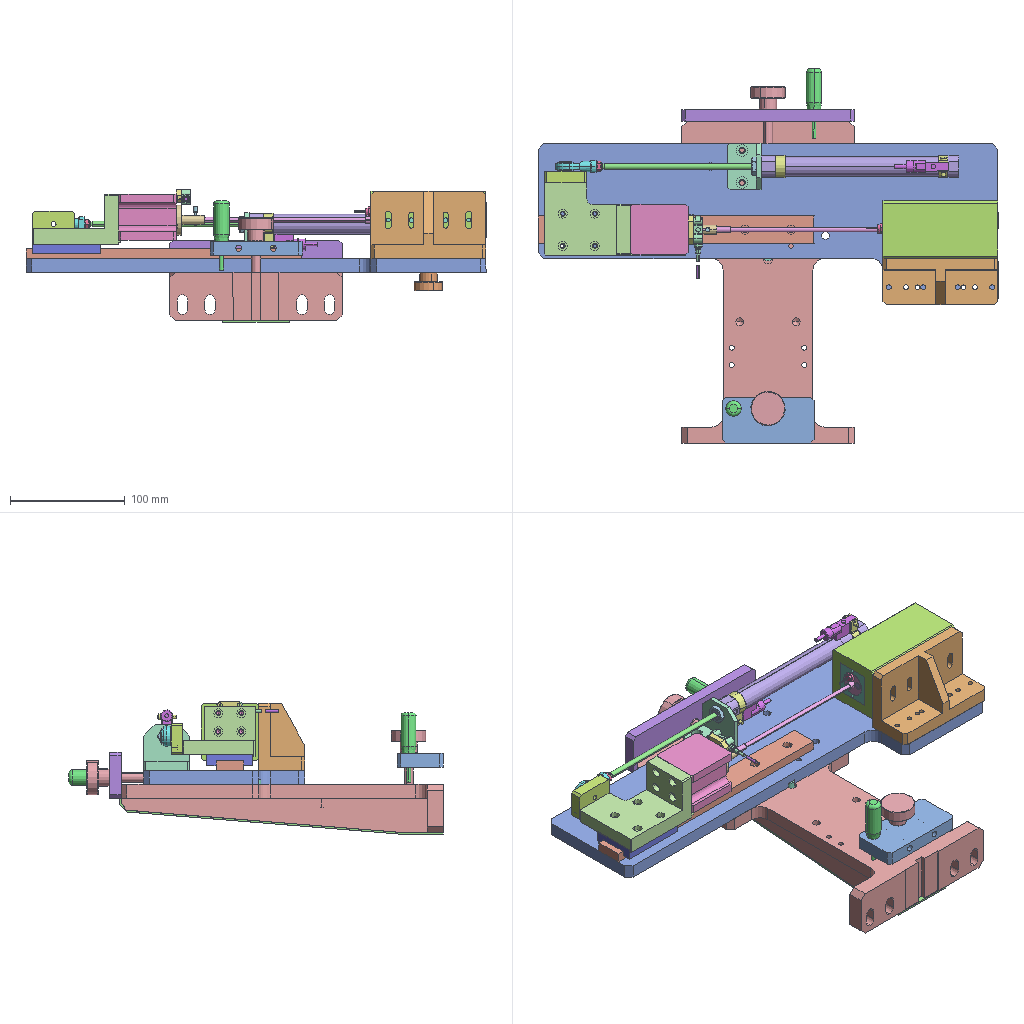Assembly | SolidWorks | 34 different items | 39 placed | box 400 x 326 x 116 mm
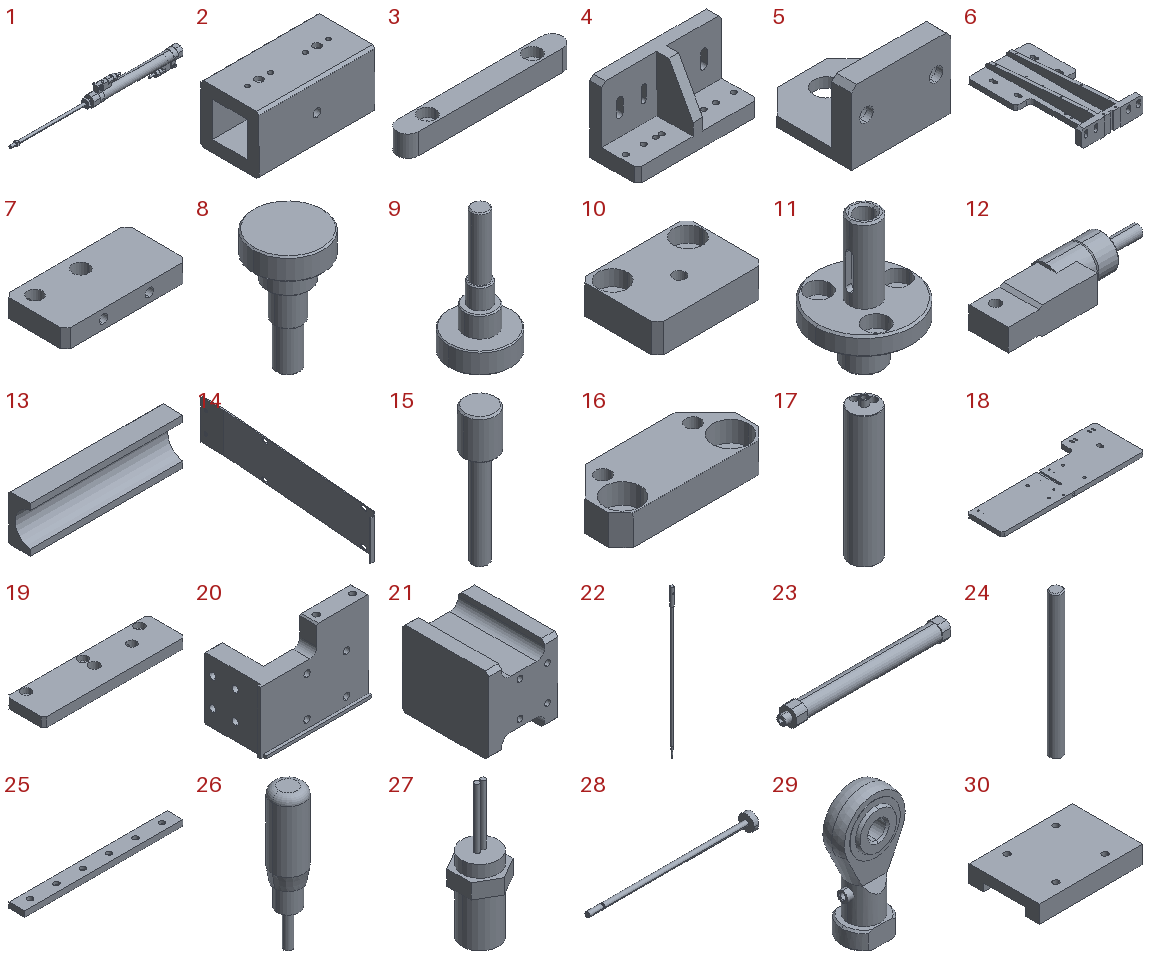Parts list (item | name | quantity | parent item | size | volume | features):
1 | (subassembly) | x1 | - | 325 x 19.2 x 45.4 mm | 28867 mm3 | -
2 | - | x1 | - | 100 x 50 x 50 mm | 157737 mm3 | features HoleWzd 7, Chamfer 1, Extrusion 1, ICE 1
3 | - | x1 | - | 63 x 8 x 8 mm | 3613 mm3 | features Extrusion 1, HoleWzd 1
4 | - | x1 | - | 100 x 40 x 58.5 mm | 98616 mm3 | features ICE 3, Chamfer 1, Extrusion 1, HoleWzd 1, Rib 1
5 | - | x1 | - | 40 x 40 x 29 mm | 12650 mm3 | features Chamfer 2, ICE 2, Extrusion 1, HoleWzd 1
6 | - | x1 | - | 150 x 280 x 42 mm | 505968 mm3 | features HoleWzd 8, ICE 7, Chamfer 3, MirrorPattern 3, Extrusion 1, Fillet 1, Rib 1
7 | - | x1 | - | 80 x 40 x 12 mm | 30513 mm3 | features HoleWzd 2, Chamfer 1, Extrusion 1, ICE 1
8 | - | x1 | - | 25 x 25 x 43 mm | 7005 mm3 | features ICE 3, Chamfer 1, Extrusion 1
9 | - | x2 | - | 30 x 30 x 60 mm | 11093 mm3 | features ICE 3, Chamfer 1, Extrusion 1
10 | - | x1 | - | 37 x 27 x 10 mm | 8705 mm3 | features HoleWzd 2, Chamfer 1, Extrusion 1
11 | - | x1 | - | 26 x 26 x 35 mm | 3387 mm3 | features ICE 4, Chamfer 1, CirPattern 1, Extrusion 1, HoleWzd 1
12 | - | x2 | in 1 | 46.7 x 14 x 10 mm | 3223 mm3 | features ICE 5, RefAxis 3, Revolution 2, 3DProfileFeature 1, Extrusion 1, RevCut 1
13 | - | x2 | - | 100 x 14 x 30 mm | 25090 mm3 | features Chamfer 1, Extrusion 1, ICE 1
14 | - | x1 | - | 31.5 x 281.5 x 58 mm | 24856 mm3 | features ICE 2, ExtruThin 1, MirrorPattern 1
15 | - | x1 | - | 4 x 4 x 17 mm | 99.928 mm3 | features Chamfer 1, Extrusion 1, ICE 1
16 | - | x1 | - | 25 x 11 x 5 mm | 959.594 mm3 | features Chamfer 2, HoleWzd 2, Extrusion 1
17 | - | x1 | - | 22 x 22 x 105 mm | 33982 mm3 | features ICE 3, Chamfer 1, Extrusion 1, HoleWzd 1
18 | - | x1 | - | 400 x 140 x 12 mm | 518070 mm3 | features HoleWzd 5, ICE 5, Chamfer 1, Extrusion 1, Fillet 1
19 | - | x1 | - | 150 x 40 x 10 mm | 56531 mm3 | features HoleWzd 3, Chamfer 1, Extrusion 1, ICE 1
20 | - | x1 | - | 77 x 44 x 63 mm | 61294 mm3 | features ICE 6, HoleWzd 4, Chamfer 1, Extrusion 1, Fillet 1
21 | - | x1 | - | 40 x 50 x 44 mm | 66825 mm3 | features HoleWzd 3, ICE 2, Chamfer 1, CirPattern 1, Extrusion 1, Fillet 1
22 | - | x1 | - | 5 x 5 x 260 mm | 2905 mm3 | features ICE 3, Chamfer 1, Extrusion 1
23 | - | x1 | in 1 | 180 x 18.3 x 18.3 mm | 16108 mm3 | features RefAxis 21, 3DProfileFeature 7, ICE 3, HoleWzd 2, RevCut 1, Revolution 1
24 | - | x1 | - | 6 x 6 x 70 mm | 1975 mm3 | features Chamfer 1, Extrusion 1
25 | - | x1 | - | 240 x 24 x 8.5 mm | 47242 mm3 | features Extrusion 1, HoleWzd 1, LPattern 1
26 | - | x2 | - | 13.5 x 13.5 x 60.5 mm | 5709 mm3 | features ICE 2, Chamfer 1, Extrusion 1, Fillet 1
27 | - | x1 | - | 7 x 8.083 x 22.5 mm | 398.885 mm3 | features ICE 3, Extrusion 1
28 | - | x1 | in 1 | 170.5 x 16 x 16 mm | 4244 mm3 | features RefAxis 9, 3DProfileFeature 3, Revolution 1
29 | - | x1 | - | 18 x 10 x 36 mm | 2766 mm3 | features Revolution 4, ICE 2, RevCut 2
30 | - | x1 | - | 59.4 x 40 x 10 mm | 17003 mm3 | features Extrusion 1, HoleWzd 1, ICE 1
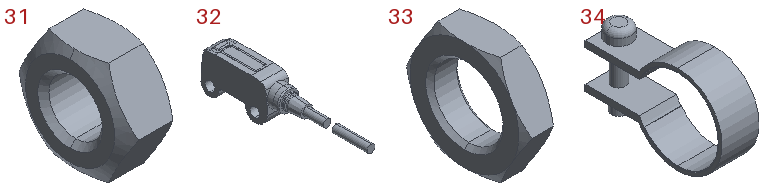31 | - | x1 | in 1 | 4 x 9.238 x 8 mm | 156.615 mm3 | features RefAxis 6, 3DProfileFeature 2, RevCut 2, Extrusion 1
32 | - | x1 | - | 7.5 x 54.319 x 13.3 mm | 2039 mm3 | features BaseBody 2
33 | - | x1 | in 1 | 4 x 16.166 x 14 mm | 414.657 mm3 | features RefAxis 6, 3DProfileFeature 2, RevCut 2, Extrusion 1
34 | - | x2 | in 1 | 8 x 29.6 x 19.2 mm | 748.959 mm3 | features RefAxis 6, 3DProfileFeature 2, Extrusion 1, ICE 1, Revolution 1
Mates (type | each side: item.copy, entity, surface, feature):
In the top assembly
Coincident | 6.1 face plane Boss-Extrude1 | 18.1 face plane Boss-Extrude1
Parallel | 6.1 face plane Boss-Extrude1 | 18.1 face plane Boss-Extrude1
Coincident | 2.1 face plane Boss-Extrude1 | 13.1 face plane Boss-Extrude1
Coincident | 2.1 face plane Cut-Extrude1 | 13.1 face plane Boss-Extrude1
Concentric | 17.1 face cylinder Boss-Extrude1 | 13.2 face cylinder Cut-Extrude1
Coincident | 17.1 face plane Boss-Extrude1 | 13.2 face plane Boss-Extrude1
Coincident | 2.1 face plane Cut-Extrude1 | 13.2 face plane Boss-Extrude1
Coincident | 18.1 face plane Boss-Extrude1 | 4.1 face plane Boss-Extrude1
Coincident | 2.1 face plane Boss-Extrude1 | 4.1 face plane Boss-Extrude1 | 3 times
Coincident | 18.1 face plane Boss-Extrude2 | 4.1 face plane Boss-Extrude1 | 2 times
Parallel | 18.1 face plane Boss-Extrude1 | 23.1 face plane Boss-Extrude1 | 3 times
Concentric | 23.1 face cylinder Revolve1 | 5.1 face cylinder Cut-Extrude1
Coincident | 18.1 face plane Boss-Extrude1 | 5.1 face plane Boss-Extrude1 | 2 times
Coincident | 23.1 face plane Boss-Extrude1 | 5.1 face plane Boss-Extrude1
Parallel | 18.1 face plane Boss-Extrude1 | 5.1 face plane Boss-Extrude1
Coincident | 18.1 face plane Boss-Extrude1 | 25.1 face plane Boss-Extrude1 | 2 times
Parallel | 18.1 face plane Boss-Extrude1 | 25.1 face plane Boss-Extrude1
Coincident | 25.1 face plane Boss-Extrude1 | 30.1 face plane Cut-Extrude1 | 3 times
Coincident | 30.1 face plane Boss-Extrude1 | 20.1 face plane Boss-Extrude1
Width | 25.1 face plane Boss-Extrude1 | 25.1 face plane Boss-Extrude1 | 30.1 face plane Boss-Extrude1 | 30.1 face plane Boss-Extrude1
Coincident | 30.1 face plane Boss-Extrude1 | 20.1 face plane Boss-Extrude2
Coincident | 20.1 face plane Boss-Extrude1 | 21.1 face plane Boss-Extrude1
Coincident | 20.1 face plane Boss-Extrude5 | 21.1 face plane Boss-Extrude1
Coincident | 20.1 face plane Cut-Extrude2 | 21.1 face plane Boss-Extrude1
Concentric | 28.1 face cylinder Revolve1 | 29.1 face cylinder Revolve1
Coincident | 31.1 face plane Boss-Extrude1 | 29.1 face plane Revolve1
DistanceDim | 5.1 face plane Boss-Extrude2 | 18.1 face plane Boss-Extrude1
Concentric | 21.1 face cylinder Cut-Extrude1 | 11.1 face cylinder Boss-Extrude1
Coincident | 21.1 face plane Boss-Extrude1 | 11.1 face plane Boss-Extrude2
Width | 6.1 face plane Boss-Extrude1 | 6.1 face plane Boss-Extrude1 | 18.1 face plane Boss-Extrude1 | 18.1 face plane Boss-Extrude1
Concentric | 21.1 face cylinder CirPattern1 | 11.1 face cylinder CirPattern1
Coincident | 6.1 face plane Boss-Extrude1 | 19.1 face plane Boss-Extrude1 | 3 times
Concentric | 19.1 face cylinder Cut-Extrude1 | 26.1 face cylinder Boss-Extrude2
Coincident | 19.1 face plane Boss-Extrude1 | 26.1 face plane Boss-Extrude3
Concentric | 19.1 face cylinder Ø10.5 (10.5) Diameter Hole1 | 9.1 face cylinder Boss-Extrude2
Coincident | 19.1 face plane Boss-Extrude1 | 9.1 face plane Boss-Extrude2
Width | 6.1 face plane Boss-Extrude1 | 6.1 face plane Boss-Extrude1 | 7.1 face plane Boss-Extrude1 | 7.1 face plane Boss-Extrude1
DistanceDim | 7.1 face plane Boss-Extrude1 | 6.1 face plane Boss-Extrude1
Concentric | 7.1 face cylinder Cut-Extrude1 | 9.2 face cylinder Boss-Extrude4
Coincident | 7.1 face plane Boss-Extrude1 | 9.2 face plane Boss-Extrude2
Concentric | 7.1 face cylinder Cut-Extrude1 | 26.2 face cylinder Boss-Extrude3
Coincident | 7.1 face plane Boss-Extrude1 | 26.2 face plane Boss-Extrude3
Coincident | 6.1 face plane Boss-Extrude1 | 7.1 face plane Boss-Extrude1
DistanceDim | 18.1 face plane Boss-Extrude1 | 6.1 face plane Boss-Extrude1
Width | 25.1 face plane Boss-Extrude1 | 25.1 face plane Boss-Extrude1 | 17.1 face cylinder Boss-Extrude2
Concentric | 20.1 face cylinder M5 Tapped Hole2 | 10.1 face cylinder CBORE for M5 Hex Socket Head Cap Screw1 | 2 times
Coincident | 20.1 face plane Cut-Extrude3 | 10.1 face plane Boss-Extrude1
Coincident | 29.1 face plane Revolve3 | 10.1 face plane Boss-Extrude1
Concentric | 29.1 face cylinder Cut-Revolve1 | 10.1 face cylinder M5 Tapped Hole1
Concentric | 11.1 face cylinder Boss-Extrude3 | 22.1 face cylinder Boss-Extrude2
Concentric | 11.1 face cylinder Cut-Extrude2 | 22.1 face cylinder Cut-Extrude1
Concentric | 30.1 face cylinder M4 Tapped Hole1 | 20.1 face cylinder CBORE for M4 Hex Socket Head Cap Screw2
Coincident | 6.1 face plane Cut-Extrude3 | 3.1 face plane Boss-Extrude1 | 2 times
Concentric | 6.1 face cylinder M3 Tapped Hole1 | 3.1 face cylinder CBORE for M3 Hex Socket Head Cap Screw1
Coincident | 2.1 face plane Boss-Extrude1 | 4.1 face plane Boss-Extrude2
Concentric | 17.1 face cylinder Boss-Extrude1 | 13.1 face cylinder Cut-Extrude1
Coincident | 2.1 face plane Boss-Extrude1 | 13.2 face plane Boss-Extrude1
Concentric | 2.1 face cylinder M8 Tapped Hole1 | 8.1 face cylinder Boss-Extrude2
Coincident | 18.1 face plane Boss-Extrude1 | 8.1 face plane Boss-Extrude3
Coincident | 6.1 face plane Boss-Extrude2 | assembly plane
Coincident | 6.1 face plane Boss-Extrude1 | assembly plane
Coincident | 6.1 face plane Mirror1 | assembly plane
Concentric | 17.1 face cylinder Cut-Extrude2 | 24.1 face cylinder Boss-Extrude1
Coincident | 17.1 face plane Boss-Extrude1 | 24.1 face plane Boss-Extrude1
Coincident | 6.1 face plane Boss-Extrude1 | 14.1 face plane Extrude-Thin2
Coincident | 6.1 face plane Boss-Extrude2 | 14.1 face plane Extrude-Thin2
Coincident | 6.1 face plane Rib1 | 14.1 face plane Extrude-Thin2
Coincident | 17.1 face plane Boss-Extrude1 | 27.1 face plane Boss-Extrude2
Concentric | 17.1 face cylinder M6 Tapped Hole1 | 27.1 face cylinder Boss-Extrude1
Concentric | 22.1 face cylinder Cut-Extrude1 | 15.1 face cylinder Boss-Extrude1
DistanceDim | 22.1 plane | 15.1 face plane Boss-Extrude1
Coincident | 21.1 face plane Boss-Extrude1 | 16.1 face plane Boss-Extrude1
Concentric | 21.1 face cylinder M3 Tapped Hole2 | 16.1 face cylinder Hole size (by socket head cap screw type)1 | 2 times
Coincident | 16.1 face plane Boss-Extrude1 | 32.1 face plane Import2
Concentric | 16.1 face cylinder M3 Tapped Hole1 | 32.1 face cylinder Import2 | 2 times
In subassembly 1
Coincident | 23.2 axis | 28.2 axis
PlanarAngleDim | 28.2 plane | 23.2 plane
LimitDistanceDim | 28.2 face plane Revolve1 | 23.2 face plane Revolve1
DistanceDim | 23.2 face plane Boss-Extrude1 | 33.1 face plane Boss-Extrude1
DistanceDim | 28.2 face plane Revolve1 | 31.2 face plane Boss-Extrude1
Concentric | 23.2 face cylinder Revolve1 | 33.1 face cylinder Cut-Revolve1
Concentric | 23.2 face cylinder Boss-Extrude2 | 34.1 face cylinder Boss-Extrude1
Parallel | 23.2 face plane Boss-Extrude3 | 12.1 face plane Boss-Extrude1
Concentric | 34.1 face cylinder Revolve1 | 12.1 face cylinder Cut-Revolve1
Coincident | 34.1 face plane Boss-Extrude1 | 12.1 face plane Boss-Extrude1
Coincident | 23.2 face plane Boss-Extrude3 | 34.1 face plane Boss-Extrude1
Concentric | 34.2 face cylinder Revolve1 | 12.2 face cylinder Cut-Revolve1
Coincident | 34.2 face plane Boss-Extrude1 | 12.2 face plane Boss-Extrude1
Parallel | 23.2 face plane Boss-Extrude1 | 12.2 face plane Boss-Extrude1
Concentric | 23.2 face cylinder Boss-Extrude2 | 34.2 face cylinder Boss-Extrude1
Coincident | 23.2 face plane Boss-Extrude1 | 12.2 face plane Boss-Extrude1